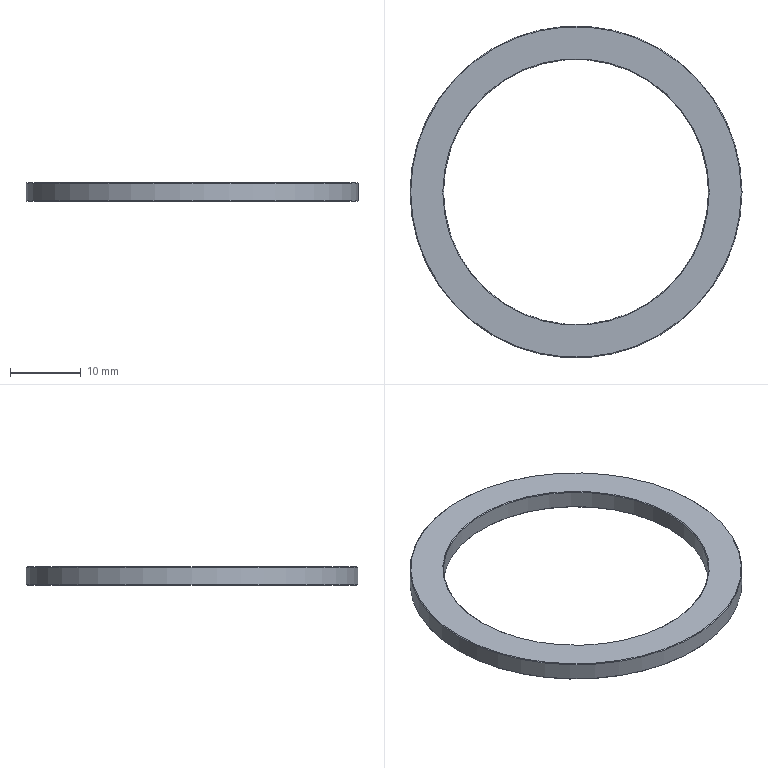Part | NX | features CHAMFER 3, DATUM_CSYS 2, EXTRUDE 1, SKETCH 1 | 1 solid | 8 faces | box 47.08 x 47.08 x 2.66 mm | volume 1678 mm3 | cone 4 | cylinder 2 | plane 2 | commonest cylinder face diameters 37.58 x1 47.08 x1
STEP:
#1=CARTESIAN_POINT('',(-23.54,0.,0.1));
#2=VERTEX_POINT('',#1);
#3=CARTESIAN_POINT('',(0.,0.,0.1));
#4=DIRECTION('',(0.,0.,-1.));
#5=DIRECTION('',(-1.,0.,0.));
#6=AXIS2_PLACEMENT_3D('',#3,#4,#5);
#7=CIRCLE('',#6,23.54);
#8=EDGE_CURVE('',#2,#2,#7,.F.);
#9=ORIENTED_EDGE('',*,*,#8,.T.);
#10=EDGE_LOOP('',(#9));
#11=FACE_BOUND('',#10,.T.);
#12=CARTESIAN_POINT('',(-23.54,0.,2.56));
#13=VERTEX_POINT('',#12);
#14=CARTESIAN_POINT('',(0.,0.,2.56));
#15=DIRECTION('',(0.,0.,-1.));
#16=DIRECTION('',(-1.,0.,0.));
#17=AXIS2_PLACEMENT_3D('',#14,#15,#16);
#18=CIRCLE('',#17,23.54);
#19=EDGE_CURVE('',#13,#13,#18,.T.);
#20=ORIENTED_EDGE('',*,*,#19,.T.);
#21=EDGE_LOOP('',(#20));
#22=FACE_BOUND('',#21,.T.);
#23=CARTESIAN_POINT('',(0.,0.,2.66));
#24=DIRECTION('',(0.,0.,-1.));
#25=DIRECTION('',(-1.,0.,0.));
#26=AXIS2_PLACEMENT_3D('',#23,#24,#25);
#27=CYLINDRICAL_SURFACE('',#26,23.54);
#28=ADVANCED_FACE('',(#11,#22),#27,.T.);
#29=CARTESIAN_POINT('',(-18.79,0.,0.1));
#30=VERTEX_POINT('',#29);
#31=CARTESIAN_POINT('',(0.,0.,0.1));
#32=DIRECTION('',(0.,0.,-1.));
#33=DIRECTION('',(-1.,0.,0.));
#34=AXIS2_PLACEMENT_3D('',#31,#32,#33);
#35=CIRCLE('',#34,18.79);
#36=EDGE_CURVE('',#30,#30,#35,.T.);
#37=ORIENTED_EDGE('',*,*,#36,.T.);
#38=EDGE_LOOP('',(#37));
#39=FACE_BOUND('',#38,.T.);
#40=CARTESIAN_POINT('',(-18.79,0.,2.56));
#41=VERTEX_POINT('',#40);
#42=CARTESIAN_POINT('',(0.,0.,2.56));
#43=DIRECTION('',(0.,0.,-1.));
#44=DIRECTION('',(-1.,0.,0.));
#45=AXIS2_PLACEMENT_3D('',#42,#43,#44);
#46=CIRCLE('',#45,18.79);
#47=EDGE_CURVE('',#41,#41,#46,.F.);
#48=ORIENTED_EDGE('',*,*,#47,.T.);
#49=EDGE_LOOP('',(#48));
#50=FACE_BOUND('',#49,.T.);
#51=CARTESIAN_POINT('',(0.,0.,2.66));
#52=DIRECTION('',(0.,0.,-1.));
#53=DIRECTION('',(-1.,0.,0.));
#54=AXIS2_PLACEMENT_3D('',#51,#52,#53);
#55=CYLINDRICAL_SURFACE('',#54,18.79);
#56=ADVANCED_FACE('',(#39,#50),#55,.F.);
#57=CARTESIAN_POINT('',(-23.44,0.,2.66));
#58=VERTEX_POINT('',#57);
#59=CARTESIAN_POINT('',(0.,0.,2.66));
#60=DIRECTION('',(0.,0.,-1.));
#61=DIRECTION('',(-1.,0.,0.));
#62=AXIS2_PLACEMENT_3D('',#59,#60,#61);
#63=CIRCLE('',#62,23.44);
#64=EDGE_CURVE('',#58,#58,#63,.F.);
#65=ORIENTED_EDGE('',*,*,#64,.T.);
#66=EDGE_LOOP('',(#65));
#67=FACE_BOUND('',#66,.T.);
#68=CARTESIAN_POINT('',(-18.89,0.,2.66));
#69=VERTEX_POINT('',#68);
#70=CARTESIAN_POINT('',(0.,0.,2.66));
#71=DIRECTION('',(0.,0.,-1.));
#72=DIRECTION('',(-1.,0.,0.));
#73=AXIS2_PLACEMENT_3D('',#70,#71,#72);
#74=CIRCLE('',#73,18.89);
#75=EDGE_CURVE('',#69,#69,#74,.T.);
#76=ORIENTED_EDGE('',*,*,#75,.T.);
#77=EDGE_LOOP('',(#76));
#78=FACE_BOUND('',#77,.T.);
#79=CARTESIAN_POINT('',(0.,0.,2.66));
#80=DIRECTION('',(0.,0.,-1.));
#81=DIRECTION('',(-1.,0.,0.));
#82=AXIS2_PLACEMENT_3D('',#79,#80,#81);
#83=PLANE('',#82);
#84=ADVANCED_FACE('',(#67,#78),#83,.F.);
#85=CARTESIAN_POINT('',(-23.44,0.,0.));
#86=VERTEX_POINT('',#85);
#87=CARTESIAN_POINT('',(0.,0.,0.));
#88=DIRECTION('',(0.,0.,-1.));
#89=DIRECTION('',(-1.,0.,0.));
#90=AXIS2_PLACEMENT_3D('',#87,#88,#89);
#91=CIRCLE('',#90,23.44);
#92=EDGE_CURVE('',#86,#86,#91,.T.);
#93=ORIENTED_EDGE('',*,*,#92,.T.);
#94=EDGE_LOOP('',(#93));
#95=FACE_BOUND('',#94,.T.);
#96=CARTESIAN_POINT('',(-18.89,0.,0.));
#97=VERTEX_POINT('',#96);
#98=CARTESIAN_POINT('',(0.,0.,0.));
#99=DIRECTION('',(0.,0.,-1.));
#100=DIRECTION('',(-1.,0.,0.));
#101=AXIS2_PLACEMENT_3D('',#98,#99,#100);
#102=CIRCLE('',#101,18.89);
#103=EDGE_CURVE('',#97,#97,#102,.F.);
#104=ORIENTED_EDGE('',*,*,#103,.T.);
#105=EDGE_LOOP('',(#104));
#106=FACE_BOUND('',#105,.T.);
#107=CARTESIAN_POINT('',(0.,0.,0.));
#108=DIRECTION('',(0.,0.,-1.));
#109=DIRECTION('',(-1.,0.,0.));
#110=AXIS2_PLACEMENT_3D('',#107,#108,#109);
#111=PLANE('',#110);
#112=ADVANCED_FACE('',(#95,#106),#111,.T.);
#113=ORIENTED_EDGE('',*,*,#103,.F.);
#114=EDGE_LOOP('',(#113));
#115=FACE_BOUND('',#114,.T.);
#116=ORIENTED_EDGE('',*,*,#36,.F.);
#117=EDGE_LOOP('',(#116));
#118=FACE_BOUND('',#117,.T.);
#119=CARTESIAN_POINT('',(0.,0.,0.1));
#120=DIRECTION('',(0.,0.,-1.));
#121=DIRECTION('',(-1.,0.,0.));
#122=AXIS2_PLACEMENT_3D('',#119,#120,#121);
#123=CONICAL_SURFACE('',#122,18.79,0.7854);
#124=ADVANCED_FACE('',(#115,#118),#123,.F.);
#125=ORIENTED_EDGE('',*,*,#47,.F.);
#126=EDGE_LOOP('',(#125));
#127=FACE_BOUND('',#126,.T.);
#128=ORIENTED_EDGE('',*,*,#75,.F.);
#129=EDGE_LOOP('',(#128));
#130=FACE_BOUND('',#129,.T.);
#131=CARTESIAN_POINT('',(0.,0.,2.66));
#132=DIRECTION('',(0.,0.,1.));
#133=DIRECTION('',(1.,0.,0.));
#134=AXIS2_PLACEMENT_3D('',#131,#132,#133);
#135=CONICAL_SURFACE('',#134,18.89,0.7854);
#136=ADVANCED_FACE('',(#127,#130),#135,.F.);
#137=ORIENTED_EDGE('',*,*,#64,.F.);
#138=EDGE_LOOP('',(#137));
#139=FACE_BOUND('',#138,.T.);
#140=ORIENTED_EDGE('',*,*,#19,.F.);
#141=EDGE_LOOP('',(#140));
#142=FACE_BOUND('',#141,.T.);
#143=CARTESIAN_POINT('',(0.,0.,2.56));
#144=DIRECTION('',(0.,0.,-1.));
#145=DIRECTION('',(-1.,0.,0.));
#146=AXIS2_PLACEMENT_3D('',#143,#144,#145);
#147=CONICAL_SURFACE('',#146,23.54,0.7854);
#148=ADVANCED_FACE('',(#139,#142),#147,.T.);
#149=ORIENTED_EDGE('',*,*,#8,.F.);
#150=EDGE_LOOP('',(#149));
#151=FACE_BOUND('',#150,.T.);
#152=ORIENTED_EDGE('',*,*,#92,.F.);
#153=EDGE_LOOP('',(#152));
#154=FACE_BOUND('',#153,.T.);
#155=CARTESIAN_POINT('',(0.,0.,0.));
#156=DIRECTION('',(0.,0.,1.));
#157=DIRECTION('',(1.,0.,0.));
#158=AXIS2_PLACEMENT_3D('',#155,#156,#157);
#159=CONICAL_SURFACE('',#158,23.44,0.7854);
#160=ADVANCED_FACE('',(#151,#154),#159,.T.);
#161=CLOSED_SHELL('',(#28,#56,#84,#112,#124,#136,#148,#160));
#162=MANIFOLD_SOLID_BREP('',#161);
#163=(LENGTH_UNIT()NAMED_UNIT(*)SI_UNIT(.MILLI.,.METRE.));
#164=UNCERTAINTY_MEASURE_WITH_UNIT(LENGTH_MEASURE(0.00001),#163,'','');
#165=(NAMED_UNIT(*)PLANE_ANGLE_UNIT()SI_UNIT($,.RADIAN.));
#166=(NAMED_UNIT(*)SI_UNIT($,.STERADIAN.)SOLID_ANGLE_UNIT());
#167=(GEOMETRIC_REPRESENTATION_CONTEXT(3)GLOBAL_UNCERTAINTY_ASSIGNED_CONTEXT((#164))GLOBAL_UNIT_ASSIGNED_CONTEXT((#163,#165,#166))REPRESENTATION_CONTEXT('',''));
#168=ADVANCED_BREP_SHAPE_REPRESENTATION('',(#162),#167);